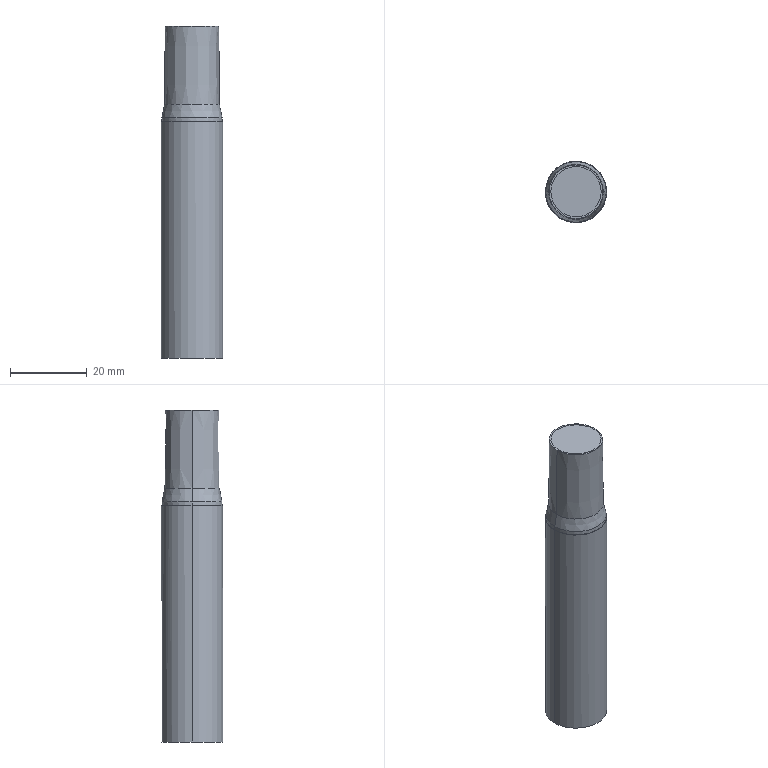Part | Creo | 1 solid | 12 faces | box 16 x 16 x 86.539 mm | volume 16401 mm3 | cylinder 4 | plane 4 | cone 4 | commonest cylinder face diameters 15.678 x2 16 x2
STEP:
#1=CARTESIAN_POINT('',(0.,0.,0.));
#2=DIRECTION('',(0.,0.,1.));
#3=DIRECTION('',(1.,0.,0.));
#4=AXIS2_PLACEMENT_3D('',#1,#2,#3);
#5=CARTESIAN_POINT('',(229.842,-56.561,-153.441));
#6=VERTEX_POINT('',#5);
#7=CARTESIAN_POINT('',(245.842,-56.561,-153.441));
#8=VERTEX_POINT('',#7);
#9=CARTESIAN_POINT('',(237.842,-56.561,-153.441));
#10=DIRECTION('',(0.,0.,-1.));
#11=DIRECTION('',(-1.,0.,0.));
#12=AXIS2_PLACEMENT_3D('',#9,#10,#11);
#13=CIRCLE('',#12,8.);
#14=EDGE_CURVE('',#6,#8,#13,.T.);
#15=ORIENTED_EDGE('',*,*,#14,.T.);
#16=CARTESIAN_POINT('',(245.842,-56.561,-91.838));
#17=VERTEX_POINT('',#16);
#18=CARTESIAN_POINT('',(245.842,-56.561,-91.838));
#19=DIRECTION('',(0.,0.,-1.));
#20=VECTOR('',#19,61.604);
#21=LINE('',#18,#20);
#22=EDGE_CURVE('',#17,#8,#21,.T.);
#23=ORIENTED_EDGE('',*,*,#22,.F.);
#24=CARTESIAN_POINT('',(229.842,-56.551,-91.817));
#25=VERTEX_POINT('',#24);
#26=CARTESIAN_POINT('',(229.843,-55.608,-91.817));
#27=CARTESIAN_POINT('',(230.187,-53.572,-91.817));
#28=CARTESIAN_POINT('',(231.716,-51.206,-91.819));
#29=CARTESIAN_POINT('',(233.444,-49.811,-91.821));
#30=CARTESIAN_POINT('',(234.894,-49.067,-91.823));
#31=CARTESIAN_POINT('',(236.146,-48.714,-91.825));
#32=CARTESIAN_POINT('',(237.132,-48.582,-91.826));
#33=CARTESIAN_POINT('',(237.847,-48.551,-91.827));
#34=CARTESIAN_POINT('',(238.561,-48.582,-91.828));
#35=CARTESIAN_POINT('',(239.547,-48.717,-91.829));
#36=CARTESIAN_POINT('',(240.799,-49.071,-91.831));
#37=CARTESIAN_POINT('',(242.248,-49.817,-91.833));
#38=CARTESIAN_POINT('',(243.974,-51.214,-91.835));
#39=CARTESIAN_POINT('',(245.5,-53.582,-91.837));
#40=CARTESIAN_POINT('',(245.842,-55.619,-91.838));
#41=B_SPLINE_CURVE_WITH_KNOTS('',3,(#24,#26,#27,#28,#29,#30,#31,#32,#33,#34,#35,#36,#37,#38,#39,#40,#16),.UNSPECIFIED.,.F.,.F.,(4,1,1,1,1,1,1,1,1,1,1,1,1,1,4),(0.,0.125,0.25,0.3125,0.375,0.4375,0.4688,0.5,0.5312,0.5625,0.625,0.6875,0.75,0.875,1.),.UNSPECIFIED.);
#42=EDGE_CURVE('',#25,#17,#41,.T.);
#43=ORIENTED_EDGE('',*,*,#42,.F.);
#44=CARTESIAN_POINT('',(229.842,-56.561,-91.817));
#45=VERTEX_POINT('',#44);
#46=CARTESIAN_POINT('',(229.842,-56.558,-91.817));
#47=CARTESIAN_POINT('',(229.842,-56.554,-91.817));
#48=CARTESIAN_POINT('',(229.842,-56.551,-91.817));
#49=B_SPLINE_CURVE_WITH_KNOTS('',3,(#44,#46,#47,#48),.UNSPECIFIED.,.F.,.F.,(4,4),(0.,1.),.UNSPECIFIED.);
#50=EDGE_CURVE('',#45,#25,#49,.T.);
#51=ORIENTED_EDGE('',*,*,#50,.F.);
#52=CARTESIAN_POINT('',(229.842,-56.561,-91.817));
#53=DIRECTION('',(-0.000000074,0.,-1.));
#54=VECTOR('',#53,61.625);
#55=LINE('',#52,#54);
#56=EDGE_CURVE('',#45,#6,#55,.T.);
#57=ORIENTED_EDGE('',*,*,#56,.T.);
#58=EDGE_LOOP('',(#15,#23,#43,#51,#57));
#59=FACE_OUTER_BOUND('',#58,.F.);
#60=CARTESIAN_POINT('',(237.842,-56.561,508.193));
#61=DIRECTION('',(0.,0.,-1.));
#62=DIRECTION('',(-1.,0.,0.));
#63=AXIS2_PLACEMENT_3D('',#60,#61,#62);
#64=CYLINDRICAL_SURFACE('',#63,8.);
#65=ADVANCED_FACE('',(#59),#64,.T.);
#66=ORIENTED_EDGE('',*,*,#14,.F.);
#67=CARTESIAN_POINT('',(237.842,-56.561,-153.441));
#68=DIRECTION('',(0.,0.,-1.));
#69=DIRECTION('',(1.,0.,0.));
#70=AXIS2_PLACEMENT_3D('',#67,#68,#69);
#71=CIRCLE('',#70,8.);
#72=EDGE_CURVE('',#8,#6,#71,.T.);
#73=ORIENTED_EDGE('',*,*,#72,.F.);
#74=EDGE_LOOP('',(#66,#73));
#75=FACE_OUTER_BOUND('',#74,.F.);
#76=CARTESIAN_POINT('',(5.725,319.968,-153.441));
#77=DIRECTION('',(0.,0.,-1.));
#78=DIRECTION('',(-1.,0.,0.));
#79=AXIS2_PLACEMENT_3D('',#76,#77,#78);
#80=PLANE('',#79);
#81=ADVANCED_FACE('',(#75),#80,.T.);
#82=ORIENTED_EDGE('',*,*,#72,.T.);
#83=ORIENTED_EDGE('',*,*,#56,.F.);
#84=CARTESIAN_POINT('',(245.842,-56.571,-91.838));
#85=VERTEX_POINT('',#84);
#86=CARTESIAN_POINT('',(245.841,-57.067,-91.838));
#87=CARTESIAN_POINT('',(245.749,-58.041,-91.838));
#88=CARTESIAN_POINT('',(245.343,-59.471,-91.837));
#89=CARTESIAN_POINT('',(244.678,-60.802,-91.836));
#90=CARTESIAN_POINT('',(243.792,-61.976,-91.835));
#91=CARTESIAN_POINT('',(242.691,-62.982,-91.834));
#92=CARTESIAN_POINT('',(241.423,-63.766,-91.832));
#93=CARTESIAN_POINT('',(240.035,-64.302,-91.83));
#94=CARTESIAN_POINT('',(238.575,-64.573,-91.828));
#95=CARTESIAN_POINT('',(237.092,-64.572,-91.826));
#96=CARTESIAN_POINT('',(235.637,-64.299,-91.824));
#97=CARTESIAN_POINT('',(234.256,-63.763,-91.822));
#98=CARTESIAN_POINT('',(232.995,-62.983,-91.821));
#99=CARTESIAN_POINT('',(231.897,-61.982,-91.819));
#100=CARTESIAN_POINT('',(231.009,-60.809,-91.818));
#101=CARTESIAN_POINT('',(230.341,-59.476,-91.817));
#102=CARTESIAN_POINT('',(229.933,-58.039,-91.817));
#103=CARTESIAN_POINT('',(229.842,-57.06,-91.817));
#104=CARTESIAN_POINT('',(229.842,-56.561,-91.817));
#105=B_SPLINE_CURVE_WITH_KNOTS('',3,(#84,#86,#87,#88,#89,#90,#91,#92,#93,#94,#95,#96,#97,#98,#99,#100,#101,#102,#103,#104),.UNSPECIFIED.,.F.,.F.,(4,1,1,1,1,1,1,1,1,1,1,1,1,1,1,1,1,4),(0.,0.05882,0.1176,0.1765,0.2353,0.2941,0.3529,0.4118,0.4706,0.5294,0.5882,0.6471,0.7059,0.7647,0.8235,0.8824,0.9412,1.),.UNSPECIFIED.);
#106=EDGE_CURVE('',#85,#45,#105,.T.);
#107=ORIENTED_EDGE('',*,*,#106,.F.);
#108=CARTESIAN_POINT('',(245.842,-56.561,-91.838));
#109=CARTESIAN_POINT('',(245.842,-56.565,-91.838));
#110=CARTESIAN_POINT('',(245.842,-56.568,-91.838));
#111=CARTESIAN_POINT('',(245.842,-56.571,-91.838));
#112=B_SPLINE_CURVE_WITH_KNOTS('',3,(#108,#109,#110,#111),.UNSPECIFIED.,.F.,.F.,(4,4),(0.,1.),.UNSPECIFIED.);
#113=EDGE_CURVE('',#17,#85,#112,.T.);
#114=ORIENTED_EDGE('',*,*,#113,.F.);
#115=ORIENTED_EDGE('',*,*,#22,.T.);
#116=EDGE_LOOP('',(#82,#83,#107,#114,#115));
#117=FACE_OUTER_BOUND('',#116,.F.);
#118=CARTESIAN_POINT('',(237.842,-56.561,508.193));
#119=DIRECTION('',(0.,0.,-1.));
#120=DIRECTION('',(-1.,0.,0.));
#121=AXIS2_PLACEMENT_3D('',#118,#119,#120);
#122=CYLINDRICAL_SURFACE('',#121,8.);
#123=ADVANCED_FACE('',(#117),#122,.T.);
#124=ORIENTED_EDGE('',*,*,#106,.T.);
#125=ORIENTED_EDGE('',*,*,#50,.T.);
#126=ORIENTED_EDGE('',*,*,#42,.T.);
#127=ORIENTED_EDGE('',*,*,#113,.T.);
#128=EDGE_LOOP('',(#124,#125,#126,#127));
#129=FACE_OUTER_BOUND('',#128,.F.);
#130=CARTESIAN_POINT('',(245.681,-56.571,-91.837));
#131=VERTEX_POINT('',#130);
#132=CARTESIAN_POINT('',(245.681,-56.561,-91.837));
#133=VERTEX_POINT('',#132);
#134=CARTESIAN_POINT('',(245.681,-56.568,-91.837));
#135=CARTESIAN_POINT('',(245.681,-56.564,-91.837));
#136=CARTESIAN_POINT('',(245.681,-56.561,-91.837));
#137=B_SPLINE_CURVE_WITH_KNOTS('',3,(#130,#134,#135,#136),.UNSPECIFIED.,.F.,.F.,(4,4),(0.,1.),.UNSPECIFIED.);
#138=EDGE_CURVE('',#131,#133,#137,.T.);
#139=ORIENTED_EDGE('',*,*,#138,.T.);
#140=CARTESIAN_POINT('',(230.003,-56.551,-91.817));
#141=VERTEX_POINT('',#140);
#142=CARTESIAN_POINT('',(245.681,-56.075,-91.837));
#143=CARTESIAN_POINT('',(245.592,-55.121,-91.837));
#144=CARTESIAN_POINT('',(245.196,-53.719,-91.837));
#145=CARTESIAN_POINT('',(244.546,-52.414,-91.836));
#146=CARTESIAN_POINT('',(243.679,-51.263,-91.835));
#147=CARTESIAN_POINT('',(242.602,-50.276,-91.833));
#148=CARTESIAN_POINT('',(241.361,-49.506,-91.832));
#149=CARTESIAN_POINT('',(240.001,-48.979,-91.83));
#150=CARTESIAN_POINT('',(238.571,-48.711,-91.828));
#151=CARTESIAN_POINT('',(237.118,-48.711,-91.826));
#152=CARTESIAN_POINT('',(235.691,-48.977,-91.824));
#153=CARTESIAN_POINT('',(234.337,-49.499,-91.823));
#154=CARTESIAN_POINT('',(233.101,-50.262,-91.821));
#155=CARTESIAN_POINT('',(232.023,-51.242,-91.819));
#156=CARTESIAN_POINT('',(231.152,-52.39,-91.818));
#157=CARTESIAN_POINT('',(230.496,-53.696,-91.817));
#158=CARTESIAN_POINT('',(230.094,-55.103,-91.817));
#159=CARTESIAN_POINT('',(230.003,-56.062,-91.817));
#160=CARTESIAN_POINT('',(230.003,-56.551,-91.817));
#161=B_SPLINE_CURVE_WITH_KNOTS('',3,(#132,#142,#143,#144,#145,#146,#147,#148,#149,#150,#151,#152,#153,#154,#155,#156,#157,#158,#159,#160),.UNSPECIFIED.,.F.,.F.,(4,1,1,1,1,1,1,1,1,1,1,1,1,1,1,1,1,4),(0.,0.05882,0.1176,0.1765,0.2353,0.2941,0.3529,0.4118,0.4706,0.5294,0.5882,0.6471,0.7059,0.7647,0.8235,0.8824,0.9412,1.),.UNSPECIFIED.);
#162=EDGE_CURVE('',#133,#141,#161,.T.);
#163=ORIENTED_EDGE('',*,*,#162,.T.);
#164=CARTESIAN_POINT('',(230.003,-56.561,-91.817));
#165=VERTEX_POINT('',#164);
#166=CARTESIAN_POINT('',(230.003,-56.554,-91.817));
#167=CARTESIAN_POINT('',(230.003,-56.558,-91.817));
#168=B_SPLINE_CURVE_WITH_KNOTS('',3,(#140,#166,#167,#164),.UNSPECIFIED.,.F.,.F.,(4,4),(0.,1.),.UNSPECIFIED.);
#169=EDGE_CURVE('',#141,#165,#168,.T.);
#170=ORIENTED_EDGE('',*,*,#169,.T.);
#171=CARTESIAN_POINT('',(230.003,-56.561,-91.817));
#172=CARTESIAN_POINT('',(230.003,-57.485,-91.817));
#173=CARTESIAN_POINT('',(230.337,-59.481,-91.817));
#174=CARTESIAN_POINT('',(231.833,-61.801,-91.819));
#175=CARTESIAN_POINT('',(233.524,-63.17,-91.821));
#176=CARTESIAN_POINT('',(234.944,-63.901,-91.823));
#177=CARTESIAN_POINT('',(236.171,-64.248,-91.825));
#178=CARTESIAN_POINT('',(237.137,-64.379,-91.826));
#179=CARTESIAN_POINT('',(237.837,-64.41,-91.827));
#180=CARTESIAN_POINT('',(238.537,-64.38,-91.828));
#181=CARTESIAN_POINT('',(239.503,-64.25,-91.829));
#182=CARTESIAN_POINT('',(240.73,-63.904,-91.831));
#183=CARTESIAN_POINT('',(242.151,-63.175,-91.833));
#184=CARTESIAN_POINT('',(243.844,-61.808,-91.835));
#185=CARTESIAN_POINT('',(245.342,-59.49,-91.837));
#186=CARTESIAN_POINT('',(245.679,-57.495,-91.837));
#187=CARTESIAN_POINT('',(245.681,-56.571,-91.837));
#188=B_SPLINE_CURVE_WITH_KNOTS('',3,(#171,#172,#173,#174,#175,#176,#177,#178,#179,#180,#181,#182,#183,#184,#185,#186,#187),.UNSPECIFIED.,.F.,.F.,(4,1,1,1,1,1,1,1,1,1,1,1,1,1,4),(0.,0.125,0.25,0.3125,0.375,0.4375,0.4688,0.5,0.5312,0.5625,0.625,0.6875,0.75,0.875,1.),.UNSPECIFIED.);
#189=EDGE_CURVE('',#165,#131,#188,.T.);
#190=ORIENTED_EDGE('',*,*,#189,.T.);
#191=EDGE_LOOP('',(#139,#163,#170,#190));
#192=FACE_BOUND('',#191,.F.);
#193=CARTESIAN_POINT('',(248.993,54.022,-91.842));
#194=DIRECTION('',(-0.001312,0.000001665,-1.));
#195=DIRECTION('',(-1.,0.,0.001312));
#196=AXIS2_PLACEMENT_3D('',#193,#194,#195);
#197=PLANE('',#196);
#198=ADVANCED_FACE('',(#129,#192),#197,.F.);
#199=CARTESIAN_POINT('',(230.001,-56.561,-90.822));
#200=VERTEX_POINT('',#199);
#201=CARTESIAN_POINT('',(245.681,-56.561,-90.822));
#202=VERTEX_POINT('',#201);
#203=CARTESIAN_POINT('',(237.84,-56.561,-90.822));
#204=DIRECTION('',(0.00002709,0.,1.));
#205=DIRECTION('',(-1.,0.,0.00002709));
#206=AXIS2_PLACEMENT_3D('',#203,#204,#205);
#207=CIRCLE('',#206,7.841);
#208=EDGE_CURVE('',#200,#202,#207,.T.);
#209=ORIENTED_EDGE('',*,*,#208,.T.);
#210=CARTESIAN_POINT('',(245.681,-56.561,-91.837));
#211=DIRECTION('',(0.0003927,0.000000008,1.));
#212=VECTOR('',#211,1.015);
#213=LINE('',#210,#212);
#214=EDGE_CURVE('',#133,#202,#213,.T.);
#215=ORIENTED_EDGE('',*,*,#214,.F.);
#216=ORIENTED_EDGE('',*,*,#138,.F.);
#217=ORIENTED_EDGE('',*,*,#189,.F.);
#218=CARTESIAN_POINT('',(230.003,-56.561,-91.817));
#219=DIRECTION('',(-0.001462,0.,1.));
#220=VECTOR('',#219,0.995);
#221=LINE('',#218,#220);
#222=EDGE_CURVE('',#165,#200,#221,.T.);
#223=ORIENTED_EDGE('',*,*,#222,.T.);
#224=EDGE_LOOP('',(#209,#215,#216,#217,#223));
#225=FACE_OUTER_BOUND('',#224,.F.);
#226=CARTESIAN_POINT('',(237.842,-56.561,-91.827));
#227=DIRECTION('',(0.,0.,1.));
#228=DIRECTION('',(1.,0.,0.));
#229=AXIS2_PLACEMENT_3D('',#226,#227,#228);
#230=CYLINDRICAL_SURFACE('',#229,7.839);
#231=ADVANCED_FACE('',(#225),#230,.T.);
#232=CARTESIAN_POINT('',(230.705,-56.561,-87.304));
#233=VERTEX_POINT('',#232);
#234=CARTESIAN_POINT('',(244.977,-56.561,-87.305));
#235=VERTEX_POINT('',#234);
#236=CARTESIAN_POINT('',(237.842,-56.561,-87.305));
#237=DIRECTION('',(0.,0.,1.));
#238=DIRECTION('',(-1.,0.,0.));
#239=AXIS2_PLACEMENT_3D('',#236,#237,#238);
#240=CIRCLE('',#239,7.136);
#241=EDGE_CURVE('',#233,#235,#240,.T.);
#242=ORIENTED_EDGE('',*,*,#241,.T.);
#243=CARTESIAN_POINT('',(244.977,-56.561,-87.305));
#244=DIRECTION('',(0.1961,0.,-0.9806));
#245=VECTOR('',#244,3.587);
#246=LINE('',#243,#245);
#247=EDGE_CURVE('',#235,#202,#246,.T.);
#248=ORIENTED_EDGE('',*,*,#247,.T.);
#249=ORIENTED_EDGE('',*,*,#208,.F.);
#250=CARTESIAN_POINT('',(230.705,-56.561,-87.304));
#251=DIRECTION('',(-0.1962,0.,-0.9806));
#252=VECTOR('',#251,3.587);
#253=LINE('',#250,#252);
#254=EDGE_CURVE('',#233,#200,#253,.T.);
#255=ORIENTED_EDGE('',*,*,#254,.F.);
#256=EDGE_LOOP('',(#242,#248,#249,#255));
#257=FACE_OUTER_BOUND('',#256,.F.);
#258=CARTESIAN_POINT('',(237.841,-56.561,-89.063));
#259=DIRECTION('',(-0.00002709,0.,-1.));
#260=DIRECTION('',(1.,0.,-0.00002709));
#261=AXIS2_PLACEMENT_3D('',#258,#259,#260);
#262=CONICAL_SURFACE('',#261,7.489,11.313);
#263=ADVANCED_FACE('',(#257),#262,.T.);
#264=ORIENTED_EDGE('',*,*,#241,.F.);
#265=CARTESIAN_POINT('',(230.848,-56.561,-66.902));
#266=VERTEX_POINT('',#265);
#267=CARTESIAN_POINT('',(230.848,-56.561,-66.902));
#268=DIRECTION('',(-0.007046,0.,-1.));
#269=VECTOR('',#268,20.403);
#270=LINE('',#267,#269);
#271=EDGE_CURVE('',#266,#233,#270,.T.);
#272=ORIENTED_EDGE('',*,*,#271,.F.);
#273=CARTESIAN_POINT('',(244.835,-56.561,-66.902));
#274=VERTEX_POINT('',#273);
#275=CARTESIAN_POINT('',(237.842,-56.561,-66.902));
#276=DIRECTION('',(0.,0.,1.));
#277=DIRECTION('',(-1.,0.,0.));
#278=AXIS2_PLACEMENT_3D('',#275,#276,#277);
#279=CIRCLE('',#278,6.993);
#280=EDGE_CURVE('',#266,#274,#279,.T.);
#281=ORIENTED_EDGE('',*,*,#280,.T.);
#282=CARTESIAN_POINT('',(244.835,-56.561,-66.902));
#283=DIRECTION('',(0.006999,0.,-1.));
#284=VECTOR('',#283,20.403);
#285=LINE('',#282,#284);
#286=EDGE_CURVE('',#274,#235,#285,.T.);
#287=ORIENTED_EDGE('',*,*,#286,.T.);
#288=EDGE_LOOP('',(#264,#272,#281,#287));
#289=FACE_OUTER_BOUND('',#288,.F.);
#290=CARTESIAN_POINT('',(237.842,-56.561,-77.103));
#291=DIRECTION('',(0.,0.,-1.));
#292=DIRECTION('',(1.,0.,0.));
#293=AXIS2_PLACEMENT_3D('',#290,#291,#292);
#294=CONICAL_SURFACE('',#293,7.064,0.4);
#295=ADVANCED_FACE('',(#289),#294,.T.);
#296=CARTESIAN_POINT('',(237.842,-56.561,-87.305));
#297=DIRECTION('',(0.,0.,1.));
#298=DIRECTION('',(1.,0.,0.));
#299=AXIS2_PLACEMENT_3D('',#296,#297,#298);
#300=CIRCLE('',#299,7.136);
#301=EDGE_CURVE('',#235,#233,#300,.T.);
#302=ORIENTED_EDGE('',*,*,#301,.F.);
#303=ORIENTED_EDGE('',*,*,#286,.F.);
#304=CARTESIAN_POINT('',(237.842,-56.561,-66.902));
#305=DIRECTION('',(0.,0.,1.));
#306=DIRECTION('',(1.,0.,0.));
#307=AXIS2_PLACEMENT_3D('',#304,#305,#306);
#308=CIRCLE('',#307,6.993);
#309=EDGE_CURVE('',#274,#266,#308,.T.);
#310=ORIENTED_EDGE('',*,*,#309,.T.);
#311=ORIENTED_EDGE('',*,*,#271,.T.);
#312=EDGE_LOOP('',(#302,#303,#310,#311));
#313=FACE_OUTER_BOUND('',#312,.F.);
#314=CARTESIAN_POINT('',(237.842,-56.561,-77.103));
#315=DIRECTION('',(0.,0.,-1.));
#316=DIRECTION('',(1.,0.,0.));
#317=AXIS2_PLACEMENT_3D('',#314,#315,#316);
#318=CONICAL_SURFACE('',#317,7.064,0.4);
#319=ADVANCED_FACE('',(#313),#318,.T.);
#320=ORIENTED_EDGE('',*,*,#301,.T.);
#321=ORIENTED_EDGE('',*,*,#254,.T.);
#322=CARTESIAN_POINT('',(237.84,-56.561,-90.822));
#323=DIRECTION('',(0.00002709,0.,1.));
#324=DIRECTION('',(1.,0.,-0.00002709));
#325=AXIS2_PLACEMENT_3D('',#322,#323,#324);
#326=CIRCLE('',#325,7.841);
#327=EDGE_CURVE('',#202,#200,#326,.T.);
#328=ORIENTED_EDGE('',*,*,#327,.F.);
#329=ORIENTED_EDGE('',*,*,#247,.F.);
#330=EDGE_LOOP('',(#320,#321,#328,#329));
#331=FACE_OUTER_BOUND('',#330,.F.);
#332=CARTESIAN_POINT('',(237.841,-56.561,-89.063));
#333=DIRECTION('',(-0.00002709,0.,-1.));
#334=DIRECTION('',(1.,0.,-0.00002709));
#335=AXIS2_PLACEMENT_3D('',#332,#333,#334);
#336=CONICAL_SURFACE('',#335,7.489,11.313);
#337=ADVANCED_FACE('',(#331),#336,.T.);
#338=ORIENTED_EDGE('',*,*,#327,.T.);
#339=ORIENTED_EDGE('',*,*,#222,.F.);
#340=ORIENTED_EDGE('',*,*,#169,.F.);
#341=ORIENTED_EDGE('',*,*,#162,.F.);
#342=ORIENTED_EDGE('',*,*,#214,.T.);
#343=EDGE_LOOP('',(#338,#339,#340,#341,#342));
#344=FACE_OUTER_BOUND('',#343,.F.);
#345=CARTESIAN_POINT('',(237.842,-56.561,-91.827));
#346=DIRECTION('',(0.,0.,1.));
#347=DIRECTION('',(1.,0.,0.));
#348=AXIS2_PLACEMENT_3D('',#345,#346,#347);
#349=CYLINDRICAL_SURFACE('',#348,7.839);
#350=ADVANCED_FACE('',(#344),#349,.T.);
#351=ORIENTED_EDGE('',*,*,#309,.F.);
#352=ORIENTED_EDGE('',*,*,#280,.F.);
#353=EDGE_LOOP('',(#351,#352));
#354=FACE_OUTER_BOUND('',#353,.F.);
#355=CARTESIAN_POINT('',(231.284,-56.561,-66.902));
#356=VERTEX_POINT('',#355);
#357=CARTESIAN_POINT('',(244.399,-56.561,-66.902));
#358=VERTEX_POINT('',#357);
#359=CARTESIAN_POINT('',(231.285,-56.995,-66.902));
#360=CARTESIAN_POINT('',(231.368,-57.846,-66.902));
#361=CARTESIAN_POINT('',(231.744,-59.089,-66.902));
#362=CARTESIAN_POINT('',(232.357,-60.232,-66.902));
#363=CARTESIAN_POINT('',(233.17,-61.222,-66.902));
#364=CARTESIAN_POINT('',(234.173,-62.048,-66.902));
#365=CARTESIAN_POINT('',(235.317,-62.659,-66.902));
#366=CARTESIAN_POINT('',(236.556,-63.034,-66.902));
#367=CARTESIAN_POINT('',(237.84,-63.16,-66.902));
#368=CARTESIAN_POINT('',(239.122,-63.035,-66.902));
#369=CARTESIAN_POINT('',(240.356,-62.663,-66.902));
#370=CARTESIAN_POINT('',(241.496,-62.057,-66.902));
#371=CARTESIAN_POINT('',(242.499,-61.236,-66.902));
#372=CARTESIAN_POINT('',(243.315,-60.247,-66.902));
#373=CARTESIAN_POINT('',(243.934,-59.101,-66.902));
#374=CARTESIAN_POINT('',(244.314,-57.852,-66.902));
#375=CARTESIAN_POINT('',(244.398,-56.998,-66.902));
#376=B_SPLINE_CURVE_WITH_KNOTS('',3,(#355,#359,#360,#361,#362,#363,#364,#365,#366,#367,#368,#369,#370,#371,#372,#373,#374,#375,#357),.UNSPECIFIED.,.F.,.F.,(4,1,1,1,1,1,1,1,1,1,1,1,1,1,1,1,4),(0.,0.0625,0.125,0.1875,0.25,0.3125,0.375,0.4375,0.5,0.5625,0.625,0.6875,0.75,0.8125,0.875,0.9375,1.),.UNSPECIFIED.);
#377=EDGE_CURVE('',#356,#358,#376,.T.);
#378=ORIENTED_EDGE('',*,*,#377,.T.);
#379=CARTESIAN_POINT('',(244.399,-56.561,-66.902));
#380=CARTESIAN_POINT('',(244.398,-56.127,-66.902));
#381=CARTESIAN_POINT('',(244.315,-55.276,-66.902));
#382=CARTESIAN_POINT('',(243.938,-54.033,-66.902));
#383=CARTESIAN_POINT('',(243.325,-52.89,-66.902));
#384=CARTESIAN_POINT('',(242.513,-51.9,-66.902));
#385=CARTESIAN_POINT('',(241.51,-51.075,-66.902));
#386=CARTESIAN_POINT('',(240.366,-50.463,-66.902));
#387=CARTESIAN_POINT('',(239.127,-50.088,-66.902));
#388=CARTESIAN_POINT('',(237.843,-49.962,-66.902));
#389=CARTESIAN_POINT('',(236.561,-50.087,-66.902));
#390=CARTESIAN_POINT('',(235.326,-50.46,-66.902));
#391=CARTESIAN_POINT('',(234.187,-51.066,-66.902));
#392=CARTESIAN_POINT('',(233.184,-51.886,-66.902));
#393=CARTESIAN_POINT('',(232.367,-52.875,-66.902));
#394=CARTESIAN_POINT('',(231.749,-54.021,-66.902));
#395=CARTESIAN_POINT('',(231.369,-55.27,-66.902));
#396=CARTESIAN_POINT('',(231.285,-56.124,-66.902));
#397=CARTESIAN_POINT('',(231.284,-56.561,-66.902));
#398=B_SPLINE_CURVE_WITH_KNOTS('',3,(#379,#380,#381,#382,#383,#384,#385,#386,#387,#388,#389,#390,#391,#392,#393,#394,#395,#396,#397),.UNSPECIFIED.,.F.,.F.,(4,1,1,1,1,1,1,1,1,1,1,1,1,1,1,1,4),(0.,0.0625,0.125,0.1875,0.25,0.3125,0.375,0.4375,0.5,0.5625,0.625,0.6875,0.75,0.8125,0.875,0.9375,1.),.UNSPECIFIED.);
#399=EDGE_CURVE('',#358,#356,#398,.T.);
#400=ORIENTED_EDGE('',*,*,#399,.T.);
#401=EDGE_LOOP('',(#378,#400));
#402=FACE_BOUND('',#401,.F.);
#403=CARTESIAN_POINT('',(237.842,-56.561,-66.902));
#404=DIRECTION('',(0.,0.,1.));
#405=DIRECTION('',(1.,0.,0.));
#406=AXIS2_PLACEMENT_3D('',#403,#404,#405);
#407=PLANE('',#406);
#408=ADVANCED_FACE('',(#354,#402),#407,.T.);
#409=ORIENTED_EDGE('',*,*,#399,.F.);
#410=ORIENTED_EDGE('',*,*,#377,.F.);
#411=EDGE_LOOP('',(#409,#410));
#412=FACE_OUTER_BOUND('',#411,.F.);
#413=CARTESIAN_POINT('',(248.542,-67.217,-66.902));
#414=DIRECTION('',(0.,0.,1.));
#415=DIRECTION('',(1.,0.,0.));
#416=AXIS2_PLACEMENT_3D('',#413,#414,#415);
#417=PLANE('',#416);
#418=ADVANCED_FACE('',(#412),#417,.T.);
#419=CLOSED_SHELL('',(#65,#81,#123,#198,#231,#263,#295,#319,#337,#350,#408,#418));
#420=MANIFOLD_SOLID_BREP('',#419);
#421=(LENGTH_UNIT()NAMED_UNIT(*)SI_UNIT(.MILLI.,.METRE.));
#422=UNCERTAINTY_MEASURE_WITH_UNIT(LENGTH_MEASURE(0.008945),#421,'','');
#423=(NAMED_UNIT(*)PLANE_ANGLE_UNIT()SI_UNIT($,.RADIAN.));
#424=PLANE_ANGLE_MEASURE_WITH_UNIT(PLANE_ANGLE_MEASURE(0.01745),#423);
#425=(CONVERSION_BASED_UNIT('DEGREE',#424)NAMED_UNIT(*)PLANE_ANGLE_UNIT());
#426=(NAMED_UNIT(*)SI_UNIT($,.STERADIAN.)SOLID_ANGLE_UNIT());
#427=(GEOMETRIC_REPRESENTATION_CONTEXT(3)GLOBAL_UNCERTAINTY_ASSIGNED_CONTEXT((#422))GLOBAL_UNIT_ASSIGNED_CONTEXT((#421,#425,#426))REPRESENTATION_CONTEXT('',''));
#428=ADVANCED_BREP_SHAPE_REPRESENTATION('',(#4,#420),#427);